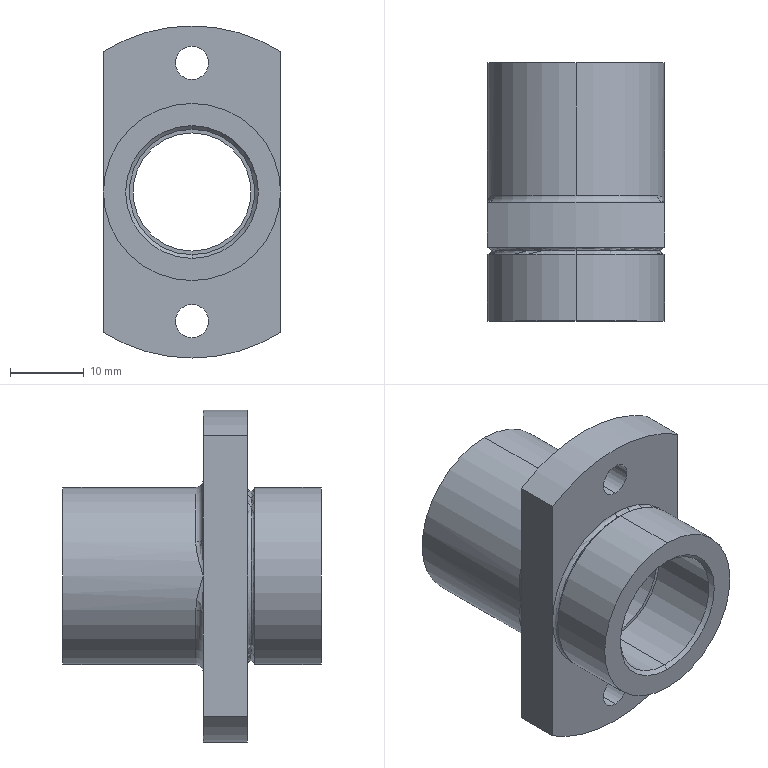Part | STEP file | 0232_214_Bushing_Holder | 1 solid | 42 faces | box 24 x 35 x 45 mm | volume 11502 mm3 | cylinder 17 | plane 10 | torus 7 | cone 4 | spline 4 | commonest cylinder face diameters 4.5 x4 17 x4 24 x4 45 x3 16 x2